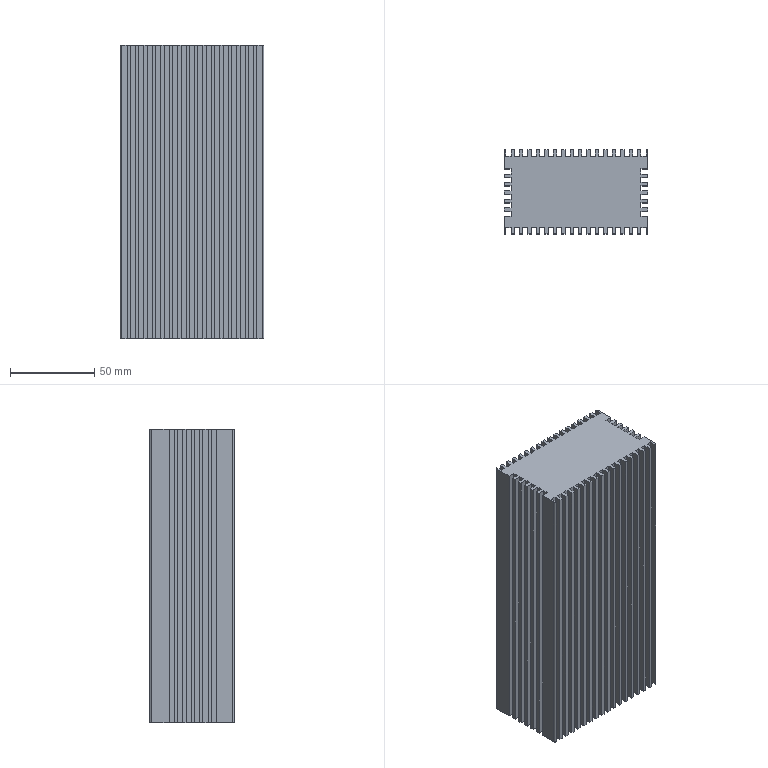Part | NX | features DATUM_CSYS 1, EXTRACT_DATUM_PLANE 1, EXTRUDE 1, SKETCH 1 | 1 solid | 190 faces | box 85 x 50 x 174 mm | volume 643303 mm3 | plane 186 | cylinder 4 | commonest cylinder face diameters 2 x4